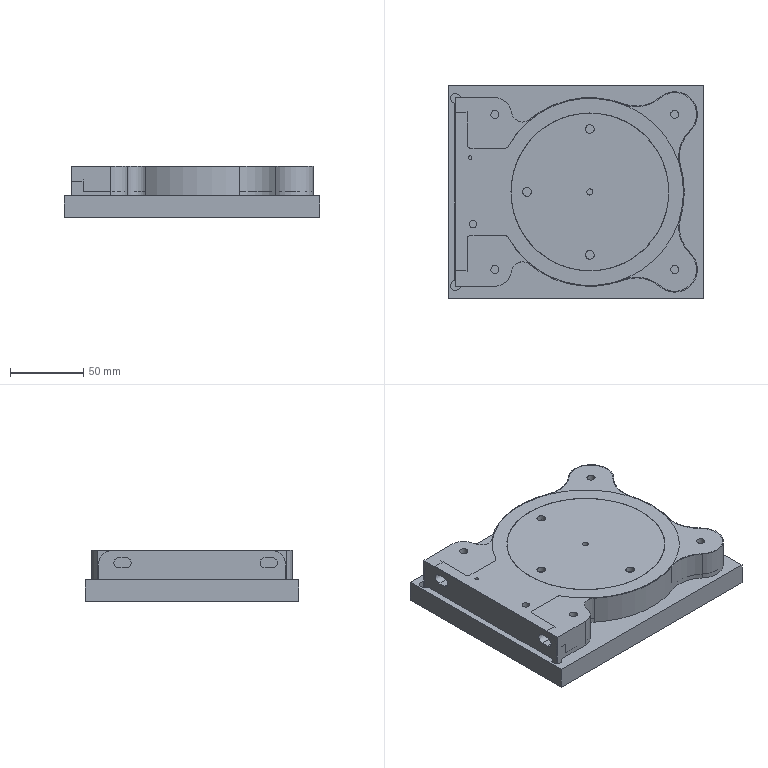Part | 13 solids | 614 faces | box 175 x 146 x 35 mm | volume 2200593 mm3 | cylinder 325 | plane 289 | commonest cylinder face diameters 4 x80 6 x36 5.5 x24 7 x24 50 x20 4.2 x12